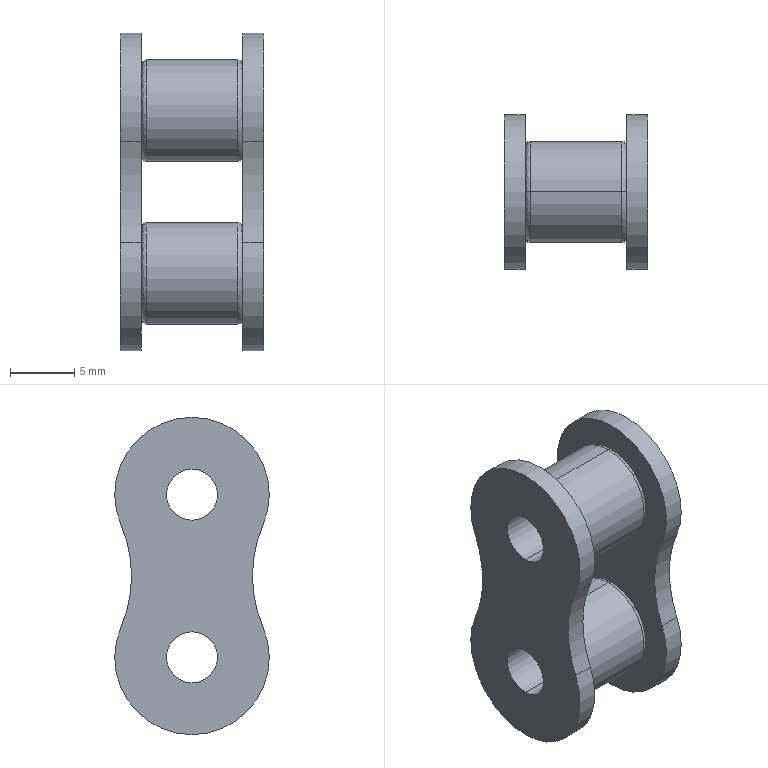Part | STEP file | 1.6 m_VMF01-40-4-A-002 | 1 solid | 30 faces | box 11.17 x 12.07 x 24.77 mm | volume 1310 mm3 | cylinder 18 | spline 8 | plane 4 | commonest cylinder face diameters 12.07 x6 3.98 x4 7.92 x4 20 x4
STEP:
#1=CARTESIAN_POINT('',(-3.56,0.,-3.96));
#2=VERTEX_POINT('',#1);
#3=CARTESIAN_POINT('',(-3.56,0.,3.96));
#4=VERTEX_POINT('',#3);
#5=CARTESIAN_POINT('',(-3.56,0.,0.));
#6=DIRECTION('',(-1.,0.,0.));
#7=DIRECTION('',(0.,0.,-1.));
#8=AXIS2_PLACEMENT_3D('',#5,#6,#7);
#9=CIRCLE('',#8,3.96);
#10=EDGE_CURVE('',#2,#4,#9,.T.);
#11=ORIENTED_EDGE('',*,*,#10,.T.);
#12=CARTESIAN_POINT('',(-3.96,0.,3.56));
#13=VERTEX_POINT('',#12);
#14=CARTESIAN_POINT('',(-3.56,0.,3.56));
#15=DIRECTION('',(0.,-1.,0.));
#16=DIRECTION('',(0.,0.,1.));
#17=AXIS2_PLACEMENT_3D('',#14,#15,#16);
#18=CIRCLE('',#17,0.4);
#19=EDGE_CURVE('',#4,#13,#18,.T.);
#20=ORIENTED_EDGE('',*,*,#19,.T.);
#21=CARTESIAN_POINT('',(-3.96,0.,-3.56));
#22=VERTEX_POINT('',#21);
#23=CARTESIAN_POINT('',(-3.96,0.,-3.56));
#24=CARTESIAN_POINT('',(-3.96,-0.2263,-3.56));
#25=CARTESIAN_POINT('',(-3.96,-0.5598,-3.529));
#26=CARTESIAN_POINT('',(-3.96,-0.9385,-3.438));
#27=CARTESIAN_POINT('',(-3.96,-1.125,-3.378));
#28=CARTESIAN_POINT('',(-3.96,-1.218,-3.345));
#29=CARTESIAN_POINT('',(-3.96,-1.258,-3.33));
#30=CARTESIAN_POINT('',(-3.96,-1.284,-3.32));
#31=CARTESIAN_POINT('',(-3.96,-1.296,-3.316));
#32=CARTESIAN_POINT('',(-3.96,-1.767,-3.129));
#33=CARTESIAN_POINT('',(-3.96,-2.17,-2.865));
#34=CARTESIAN_POINT('',(-3.96,-2.691,-2.344));
#35=CARTESIAN_POINT('',(-3.96,-2.92,-2.063));
#36=CARTESIAN_POINT('',(-3.96,-3.133,-1.699));
#37=CARTESIAN_POINT('',(-3.96,-3.226,-1.507));
#38=CARTESIAN_POINT('',(-3.96,-3.269,-1.41));
#39=CARTESIAN_POINT('',(-3.96,-3.287,-1.367));
#40=CARTESIAN_POINT('',(-3.96,-3.299,-1.339));
#41=CARTESIAN_POINT('',(-3.96,-3.305,-1.324));
#42=CARTESIAN_POINT('',(-3.96,-3.477,-0.8899));
#43=CARTESIAN_POINT('',(-3.96,-3.56,-0.4523));
#44=CARTESIAN_POINT('',(-3.96,-3.56,0.2262));
#45=CARTESIAN_POINT('',(-3.96,-3.529,0.5596));
#46=CARTESIAN_POINT('',(-3.96,-3.438,0.9384));
#47=CARTESIAN_POINT('',(-3.96,-3.378,1.125));
#48=CARTESIAN_POINT('',(-3.96,-3.345,1.218));
#49=CARTESIAN_POINT('',(-3.96,-3.33,1.258));
#50=CARTESIAN_POINT('',(-3.96,-3.32,1.284));
#51=CARTESIAN_POINT('',(-3.96,-3.316,1.296));
#52=CARTESIAN_POINT('',(-3.96,-3.129,1.767));
#53=CARTESIAN_POINT('',(-3.96,-2.865,2.17));
#54=CARTESIAN_POINT('',(-3.96,-2.344,2.691));
#55=CARTESIAN_POINT('',(-3.96,-2.063,2.92));
#56=CARTESIAN_POINT('',(-3.96,-1.699,3.133));
#57=CARTESIAN_POINT('',(-3.96,-1.507,3.226));
#58=CARTESIAN_POINT('',(-3.96,-1.41,3.269));
#59=CARTESIAN_POINT('',(-3.96,-1.367,3.287));
#60=CARTESIAN_POINT('',(-3.96,-1.339,3.299));
#61=CARTESIAN_POINT('',(-3.96,-1.324,3.305));
#62=CARTESIAN_POINT('',(-3.96,-0.8899,3.477));
#63=CARTESIAN_POINT('',(-3.96,-0.4523,3.56));
#64=CARTESIAN_POINT('',(-3.96,0.,3.56));
#65=B_SPLINE_CURVE_WITH_KNOTS('',3,(#23,#24,#25,#26,#27,#28,#29,#30,#31,#32,#33,#34,#35,#36,#37,#38,#39,#40,#41,#42,#43,#44,#45,#46,#47,#48,#49,#50,#51,#52,#53,#54,#55,#56,#57,#58,#59,#60,#61,#62,#63,#64),.UNSPECIFIED.,.F.,.F.,(4,1,1,1,1,2,2,2,1,1,1,1,2,2,2,1,1,1,1,2,2,2,1,1,1,1,2,2,4),(0.,0.03125,0.04687,0.05469,0.05859,0.06055,0.0625,0.125,0.1562,0.1719,0.1797,0.1836,0.1855,0.1875,0.25,0.2813,0.2969,0.3047,0.3086,0.3105,0.3125,0.375,0.4063,0.4219,0.4297,0.4336,0.4355,0.4375,0.5),.UNSPECIFIED.);
#66=EDGE_CURVE('',#22,#13,#65,.T.);
#67=ORIENTED_EDGE('',*,*,#66,.F.);
#68=CARTESIAN_POINT('',(-3.56,0.,-3.56));
#69=DIRECTION('',(0.,1.,0.));
#70=DIRECTION('',(0.,0.,-1.));
#71=AXIS2_PLACEMENT_3D('',#68,#69,#70);
#72=CIRCLE('',#71,0.4);
#73=EDGE_CURVE('',#2,#22,#72,.T.);
#74=ORIENTED_EDGE('',*,*,#73,.F.);
#75=EDGE_LOOP('',(#11,#20,#67,#74));
#76=FACE_OUTER_BOUND('',#75,.T.);
#77=CARTESIAN_POINT('',(-3.56,0.,3.96));
#78=CARTESIAN_POINT('',(-3.56,-7.92,3.96));
#79=CARTESIAN_POINT('',(-3.56,-7.92,-3.96));
#80=CARTESIAN_POINT('',(-3.56,0.,-3.96));
#81=CARTESIAN_POINT('',(-3.794,0.,3.96));
#82=CARTESIAN_POINT('',(-3.794,-7.92,3.96));
#83=CARTESIAN_POINT('',(-3.794,-7.92,-3.96));
#84=CARTESIAN_POINT('',(-3.794,0.,-3.96));
#85=CARTESIAN_POINT('',(-3.96,0.,3.794));
#86=CARTESIAN_POINT('',(-3.96,-7.589,3.794));
#87=CARTESIAN_POINT('',(-3.96,-7.589,-3.794));
#88=CARTESIAN_POINT('',(-3.96,0.,-3.794));
#89=CARTESIAN_POINT('',(-3.96,0.,3.56));
#90=CARTESIAN_POINT('',(-3.96,-7.12,3.56));
#91=CARTESIAN_POINT('',(-3.96,-7.12,-3.56));
#92=CARTESIAN_POINT('',(-3.96,0.,-3.56));
#93=(BOUNDED_SURFACE()B_SPLINE_SURFACE(3,3,((#77,#78,#79,#80),(#81,#82,#83,#84),(#85,#86,#87,#88),(#89,#90,#91,#92)),.UNSPECIFIED.,.F.,.F.,.F.)B_SPLINE_SURFACE_WITH_KNOTS((4,4),(4,4),(0.,1.),(0.,1.),.UNSPECIFIED.)GEOMETRIC_REPRESENTATION_ITEM()RATIONAL_B_SPLINE_SURFACE(((1.,0.3333,0.3333,1.),(0.8047,0.2682,0.2682,0.8047),(0.8047,0.2682,0.2682,0.8047),(1.,0.3333,0.3333,1.)))REPRESENTATION_ITEM('')SURFACE());
#94=ADVANCED_FACE('',(#76),#93,.T.);
#95=CARTESIAN_POINT('',(-3.56,0.,-16.66));
#96=VERTEX_POINT('',#95);
#97=CARTESIAN_POINT('',(-3.56,0.,-8.74));
#98=VERTEX_POINT('',#97);
#99=CARTESIAN_POINT('',(-3.56,0.,-12.7));
#100=DIRECTION('',(-1.,0.,0.));
#101=DIRECTION('',(0.,0.,-1.));
#102=AXIS2_PLACEMENT_3D('',#99,#100,#101);
#103=CIRCLE('',#102,3.96);
#104=EDGE_CURVE('',#96,#98,#103,.T.);
#105=ORIENTED_EDGE('',*,*,#104,.T.);
#106=CARTESIAN_POINT('',(-3.96,0.,-9.14));
#107=VERTEX_POINT('',#106);
#108=CARTESIAN_POINT('',(-3.56,0.,-9.14));
#109=DIRECTION('',(0.,-1.,0.));
#110=DIRECTION('',(0.,0.,1.));
#111=AXIS2_PLACEMENT_3D('',#108,#109,#110);
#112=CIRCLE('',#111,0.4);
#113=EDGE_CURVE('',#98,#107,#112,.T.);
#114=ORIENTED_EDGE('',*,*,#113,.T.);
#115=CARTESIAN_POINT('',(-3.96,0.,-16.26));
#116=VERTEX_POINT('',#115);
#117=CARTESIAN_POINT('',(-3.96,0.,-16.26));
#118=CARTESIAN_POINT('',(-3.96,-0.2263,-16.26));
#119=CARTESIAN_POINT('',(-3.96,-0.5598,-16.229));
#120=CARTESIAN_POINT('',(-3.96,-0.9385,-16.138));
#121=CARTESIAN_POINT('',(-3.96,-1.125,-16.078));
#122=CARTESIAN_POINT('',(-3.96,-1.218,-16.045));
#123=CARTESIAN_POINT('',(-3.96,-1.258,-16.03));
#124=CARTESIAN_POINT('',(-3.96,-1.284,-16.02));
#125=CARTESIAN_POINT('',(-3.96,-1.296,-16.016));
#126=CARTESIAN_POINT('',(-3.96,-1.767,-15.829));
#127=CARTESIAN_POINT('',(-3.96,-2.17,-15.565));
#128=CARTESIAN_POINT('',(-3.96,-2.691,-15.044));
#129=CARTESIAN_POINT('',(-3.96,-2.92,-14.763));
#130=CARTESIAN_POINT('',(-3.96,-3.133,-14.399));
#131=CARTESIAN_POINT('',(-3.96,-3.226,-14.207));
#132=CARTESIAN_POINT('',(-3.96,-3.269,-14.11));
#133=CARTESIAN_POINT('',(-3.96,-3.287,-14.067));
#134=CARTESIAN_POINT('',(-3.96,-3.299,-14.039));
#135=CARTESIAN_POINT('',(-3.96,-3.305,-14.024));
#136=CARTESIAN_POINT('',(-3.96,-3.477,-13.59));
#137=CARTESIAN_POINT('',(-3.96,-3.56,-13.152));
#138=CARTESIAN_POINT('',(-3.96,-3.56,-12.474));
#139=CARTESIAN_POINT('',(-3.96,-3.529,-12.14));
#140=CARTESIAN_POINT('',(-3.96,-3.438,-11.762));
#141=CARTESIAN_POINT('',(-3.96,-3.378,-11.575));
#142=CARTESIAN_POINT('',(-3.96,-3.345,-11.482));
#143=CARTESIAN_POINT('',(-3.96,-3.33,-11.442));
#144=CARTESIAN_POINT('',(-3.96,-3.32,-11.416));
#145=CARTESIAN_POINT('',(-3.96,-3.316,-11.404));
#146=CARTESIAN_POINT('',(-3.96,-3.129,-10.933));
#147=CARTESIAN_POINT('',(-3.96,-2.865,-10.53));
#148=CARTESIAN_POINT('',(-3.96,-2.344,-10.009));
#149=CARTESIAN_POINT('',(-3.96,-2.063,-9.78));
#150=CARTESIAN_POINT('',(-3.96,-1.699,-9.567));
#151=CARTESIAN_POINT('',(-3.96,-1.507,-9.474));
#152=CARTESIAN_POINT('',(-3.96,-1.41,-9.431));
#153=CARTESIAN_POINT('',(-3.96,-1.367,-9.413));
#154=CARTESIAN_POINT('',(-3.96,-1.339,-9.401));
#155=CARTESIAN_POINT('',(-3.96,-1.324,-9.395));
#156=CARTESIAN_POINT('',(-3.96,-0.8899,-9.223));
#157=CARTESIAN_POINT('',(-3.96,-0.4523,-9.14));
#158=CARTESIAN_POINT('',(-3.96,0.,-9.14));
#159=B_SPLINE_CURVE_WITH_KNOTS('',3,(#117,#118,#119,#120,#121,#122,#123,#124,#125,#126,#127,#128,#129,#130,#131,#132,#133,#134,#135,#136,#137,#138,#139,#140,#141,#142,#143,#144,#145,#146,#147,#148,#149,#150,#151,#152,#153,#154,#155,#156,#157,#158),.UNSPECIFIED.,.F.,.F.,(4,1,1,1,1,2,2,2,1,1,1,1,2,2,2,1,1,1,1,2,2,2,1,1,1,1,2,2,4),(0.,0.03125,0.04688,0.05469,0.05859,0.06055,0.0625,0.125,0.1562,0.1719,0.1797,0.1836,0.1855,0.1875,0.25,0.2812,0.2969,0.3047,0.3086,0.3105,0.3125,0.375,0.4062,0.4219,0.4297,0.4336,0.4355,0.4375,0.5),.UNSPECIFIED.);
#160=EDGE_CURVE('',#116,#107,#159,.T.);
#161=ORIENTED_EDGE('',*,*,#160,.F.);
#162=CARTESIAN_POINT('',(-3.56,0.,-16.26));
#163=DIRECTION('',(0.,1.,0.));
#164=DIRECTION('',(0.,0.,-1.));
#165=AXIS2_PLACEMENT_3D('',#162,#163,#164);
#166=CIRCLE('',#165,0.4);
#167=EDGE_CURVE('',#96,#116,#166,.T.);
#168=ORIENTED_EDGE('',*,*,#167,.F.);
#169=EDGE_LOOP('',(#105,#114,#161,#168));
#170=FACE_OUTER_BOUND('',#169,.T.);
#171=CARTESIAN_POINT('',(-3.56,0.,-8.74));
#172=CARTESIAN_POINT('',(-3.56,-7.92,-8.74));
#173=CARTESIAN_POINT('',(-3.56,-7.92,-16.66));
#174=CARTESIAN_POINT('',(-3.56,0.,-16.66));
#175=CARTESIAN_POINT('',(-3.794,0.,-8.74));
#176=CARTESIAN_POINT('',(-3.794,-7.92,-8.74));
#177=CARTESIAN_POINT('',(-3.794,-7.92,-16.66));
#178=CARTESIAN_POINT('',(-3.794,0.,-16.66));
#179=CARTESIAN_POINT('',(-3.96,0.,-8.906));
#180=CARTESIAN_POINT('',(-3.96,-7.589,-8.906));
#181=CARTESIAN_POINT('',(-3.96,-7.589,-16.494));
#182=CARTESIAN_POINT('',(-3.96,0.,-16.494));
#183=CARTESIAN_POINT('',(-3.96,0.,-9.14));
#184=CARTESIAN_POINT('',(-3.96,-7.12,-9.14));
#185=CARTESIAN_POINT('',(-3.96,-7.12,-16.26));
#186=CARTESIAN_POINT('',(-3.96,0.,-16.26));
#187=(BOUNDED_SURFACE()B_SPLINE_SURFACE(3,3,((#171,#172,#173,#174),(#175,#176,#177,#178),(#179,#180,#181,#182),(#183,#184,#185,#186)),.UNSPECIFIED.,.F.,.F.,.F.)B_SPLINE_SURFACE_WITH_KNOTS((4,4),(4,4),(0.,1.),(0.,1.),.UNSPECIFIED.)GEOMETRIC_REPRESENTATION_ITEM()RATIONAL_B_SPLINE_SURFACE(((1.,0.3333,0.3333,1.),(0.8047,0.2682,0.2682,0.8047),(0.8047,0.2682,0.2682,0.8047),(1.,0.3333,0.3333,1.)))REPRESENTATION_ITEM('')SURFACE());
#188=ADVANCED_FACE('',(#170),#187,.T.);
#189=CARTESIAN_POINT('',(3.96,0.,-3.56));
#190=VERTEX_POINT('',#189);
#191=CARTESIAN_POINT('',(3.96,0.,3.56));
#192=VERTEX_POINT('',#191);
#193=CARTESIAN_POINT('',(3.96,0.,-3.56));
#194=CARTESIAN_POINT('',(3.96,-7.12,-3.56));
#195=CARTESIAN_POINT('',(3.96,-7.12,3.56));
#196=CARTESIAN_POINT('',(3.96,0.,3.56));
#197=(BOUNDED_CURVE()B_SPLINE_CURVE(3,(#193,#194,#195,#196),.UNSPECIFIED.,.F.,.F.)B_SPLINE_CURVE_WITH_KNOTS((4,4),(0.,0.5),.UNSPECIFIED.)CURVE()GEOMETRIC_REPRESENTATION_ITEM()RATIONAL_B_SPLINE_CURVE((1.,0.3333,0.3333,1.))REPRESENTATION_ITEM(''));
#198=EDGE_CURVE('',#190,#192,#197,.T.);
#199=ORIENTED_EDGE('',*,*,#198,.T.);
#200=CARTESIAN_POINT('',(3.56,0.,3.96));
#201=VERTEX_POINT('',#200);
#202=CARTESIAN_POINT('',(3.56,0.,3.56));
#203=DIRECTION('',(0.,-1.,0.));
#204=DIRECTION('',(0.,0.,1.));
#205=AXIS2_PLACEMENT_3D('',#202,#203,#204);
#206=CIRCLE('',#205,0.4);
#207=EDGE_CURVE('',#192,#201,#206,.T.);
#208=ORIENTED_EDGE('',*,*,#207,.T.);
#209=CARTESIAN_POINT('',(3.56,0.,-3.96));
#210=VERTEX_POINT('',#209);
#211=CARTESIAN_POINT('',(3.56,0.,0.));
#212=DIRECTION('',(-1.,0.,0.));
#213=DIRECTION('',(0.,0.,1.));
#214=AXIS2_PLACEMENT_3D('',#211,#212,#213);
#215=CIRCLE('',#214,3.96);
#216=EDGE_CURVE('',#210,#201,#215,.T.);
#217=ORIENTED_EDGE('',*,*,#216,.F.);
#218=CARTESIAN_POINT('',(3.56,0.,-3.56));
#219=DIRECTION('',(0.,1.,0.));
#220=DIRECTION('',(0.,0.,-1.));
#221=AXIS2_PLACEMENT_3D('',#218,#219,#220);
#222=CIRCLE('',#221,0.4);
#223=EDGE_CURVE('',#190,#210,#222,.T.);
#224=ORIENTED_EDGE('',*,*,#223,.F.);
#225=EDGE_LOOP('',(#199,#208,#217,#224));
#226=FACE_OUTER_BOUND('',#225,.T.);
#227=CARTESIAN_POINT('',(3.96,0.,3.56));
#228=CARTESIAN_POINT('',(3.96,-7.12,3.56));
#229=CARTESIAN_POINT('',(3.96,-7.12,-3.56));
#230=CARTESIAN_POINT('',(3.96,0.,-3.56));
#231=CARTESIAN_POINT('',(3.96,0.,3.794));
#232=CARTESIAN_POINT('',(3.96,-7.589,3.794));
#233=CARTESIAN_POINT('',(3.96,-7.589,-3.794));
#234=CARTESIAN_POINT('',(3.96,0.,-3.794));
#235=CARTESIAN_POINT('',(3.794,0.,3.96));
#236=CARTESIAN_POINT('',(3.794,-7.92,3.96));
#237=CARTESIAN_POINT('',(3.794,-7.92,-3.96));
#238=CARTESIAN_POINT('',(3.794,0.,-3.96));
#239=CARTESIAN_POINT('',(3.56,0.,3.96));
#240=CARTESIAN_POINT('',(3.56,-7.92,3.96));
#241=CARTESIAN_POINT('',(3.56,-7.92,-3.96));
#242=CARTESIAN_POINT('',(3.56,0.,-3.96));
#243=(BOUNDED_SURFACE()B_SPLINE_SURFACE(3,3,((#227,#228,#229,#230),(#231,#232,#233,#234),(#235,#236,#237,#238),(#239,#240,#241,#242)),.UNSPECIFIED.,.F.,.F.,.F.)B_SPLINE_SURFACE_WITH_KNOTS((4,4),(4,4),(0.,1.),(0.,1.),.UNSPECIFIED.)GEOMETRIC_REPRESENTATION_ITEM()RATIONAL_B_SPLINE_SURFACE(((1.,0.3333,0.3333,1.),(0.8047,0.2682,0.2682,0.8047),(0.8047,0.2682,0.2682,0.8047),(1.,0.3333,0.3333,1.)))REPRESENTATION_ITEM('')SURFACE());
#244=ADVANCED_FACE('',(#226),#243,.T.);
#245=CARTESIAN_POINT('',(3.96,0.,-16.26));
#246=VERTEX_POINT('',#245);
#247=CARTESIAN_POINT('',(3.96,0.,-9.14));
#248=VERTEX_POINT('',#247);
#249=CARTESIAN_POINT('',(3.96,0.,-16.26));
#250=CARTESIAN_POINT('',(3.96,-7.12,-16.26));
#251=CARTESIAN_POINT('',(3.96,-7.12,-9.14));
#252=CARTESIAN_POINT('',(3.96,0.,-9.14));
#253=(BOUNDED_CURVE()B_SPLINE_CURVE(3,(#249,#250,#251,#252),.UNSPECIFIED.,.F.,.F.)B_SPLINE_CURVE_WITH_KNOTS((4,4),(0.,0.5),.UNSPECIFIED.)CURVE()GEOMETRIC_REPRESENTATION_ITEM()RATIONAL_B_SPLINE_CURVE((1.,0.3333,0.3333,1.))REPRESENTATION_ITEM(''));
#254=EDGE_CURVE('',#246,#248,#253,.T.);
#255=ORIENTED_EDGE('',*,*,#254,.T.);
#256=CARTESIAN_POINT('',(3.56,0.,-8.74));
#257=VERTEX_POINT('',#256);
#258=CARTESIAN_POINT('',(3.56,0.,-9.14));
#259=DIRECTION('',(0.,-1.,0.));
#260=DIRECTION('',(0.,0.,1.));
#261=AXIS2_PLACEMENT_3D('',#258,#259,#260);
#262=CIRCLE('',#261,0.4);
#263=EDGE_CURVE('',#248,#257,#262,.T.);
#264=ORIENTED_EDGE('',*,*,#263,.T.);
#265=CARTESIAN_POINT('',(3.56,0.,-16.66));
#266=VERTEX_POINT('',#265);
#267=CARTESIAN_POINT('',(3.56,0.,-12.7));
#268=DIRECTION('',(-1.,0.,0.));
#269=DIRECTION('',(0.,0.,1.));
#270=AXIS2_PLACEMENT_3D('',#267,#268,#269);
#271=CIRCLE('',#270,3.96);
#272=EDGE_CURVE('',#266,#257,#271,.T.);
#273=ORIENTED_EDGE('',*,*,#272,.F.);
#274=CARTESIAN_POINT('',(3.56,0.,-16.26));
#275=DIRECTION('',(0.,1.,0.));
#276=DIRECTION('',(0.,0.,-1.));
#277=AXIS2_PLACEMENT_3D('',#274,#275,#276);
#278=CIRCLE('',#277,0.4);
#279=EDGE_CURVE('',#246,#266,#278,.T.);
#280=ORIENTED_EDGE('',*,*,#279,.F.);
#281=EDGE_LOOP('',(#255,#264,#273,#280));
#282=FACE_OUTER_BOUND('',#281,.T.);
#283=CARTESIAN_POINT('',(3.96,0.,-9.14));
#284=CARTESIAN_POINT('',(3.96,-7.12,-9.14));
#285=CARTESIAN_POINT('',(3.96,-7.12,-16.26));
#286=CARTESIAN_POINT('',(3.96,0.,-16.26));
#287=CARTESIAN_POINT('',(3.96,0.,-8.906));
#288=CARTESIAN_POINT('',(3.96,-7.589,-8.906));
#289=CARTESIAN_POINT('',(3.96,-7.589,-16.494));
#290=CARTESIAN_POINT('',(3.96,0.,-16.494));
#291=CARTESIAN_POINT('',(3.794,0.,-8.74));
#292=CARTESIAN_POINT('',(3.794,-7.92,-8.74));
#293=CARTESIAN_POINT('',(3.794,-7.92,-16.66));
#294=CARTESIAN_POINT('',(3.794,0.,-16.66));
#295=CARTESIAN_POINT('',(3.56,0.,-8.74));
#296=CARTESIAN_POINT('',(3.56,-7.92,-8.74));
#297=CARTESIAN_POINT('',(3.56,-7.92,-16.66));
#298=CARTESIAN_POINT('',(3.56,0.,-16.66));
#299=(BOUNDED_SURFACE()B_SPLINE_SURFACE(3,3,((#283,#284,#285,#286),(#287,#288,#289,#290),(#291,#292,#293,#294),(#295,#296,#297,#298)),.UNSPECIFIED.,.F.,.F.,.F.)B_SPLINE_SURFACE_WITH_KNOTS((4,4),(4,4),(0.,1.),(0.,1.),.UNSPECIFIED.)GEOMETRIC_REPRESENTATION_ITEM()RATIONAL_B_SPLINE_SURFACE(((1.,0.3333,0.3333,1.),(0.8047,0.2682,0.2682,0.8047),(0.8047,0.2682,0.2682,0.8047),(1.,0.3333,0.3333,1.)))REPRESENTATION_ITEM('')SURFACE());
#300=ADVANCED_FACE('',(#282),#299,.T.);
#301=CARTESIAN_POINT('',(-5.585,0.,-1.99));
#302=VERTEX_POINT('',#301);
#303=CARTESIAN_POINT('',(-5.585,0.,1.99));
#304=VERTEX_POINT('',#303);
#305=CARTESIAN_POINT('',(-5.585,0.,0.));
#306=DIRECTION('',(-1.,0.,0.));
#307=DIRECTION('',(0.,0.,-1.));
#308=AXIS2_PLACEMENT_3D('',#305,#306,#307);
#309=CIRCLE('',#308,1.99);
#310=EDGE_CURVE('',#302,#304,#309,.T.);
#311=ORIENTED_EDGE('',*,*,#310,.T.);
#312=CARTESIAN_POINT('',(5.585,0.,1.99));
#313=VERTEX_POINT('',#312);
#314=CARTESIAN_POINT('',(5.585,0.,1.99));
#315=DIRECTION('',(1.,0.,0.));
#316=VECTOR('',#315,1000.);
#317=LINE('',#314,#316);
#318=EDGE_CURVE('',#304,#313,#317,.T.);
#319=ORIENTED_EDGE('',*,*,#318,.T.);
#320=CARTESIAN_POINT('',(5.585,0.,-1.99));
#321=VERTEX_POINT('',#320);
#322=CARTESIAN_POINT('',(5.585,0.,0.));
#323=DIRECTION('',(-1.,0.,0.));
#324=DIRECTION('',(0.,0.,-1.));
#325=AXIS2_PLACEMENT_3D('',#322,#323,#324);
#326=CIRCLE('',#325,1.99);
#327=EDGE_CURVE('',#321,#313,#326,.T.);
#328=ORIENTED_EDGE('',*,*,#327,.F.);
#329=CARTESIAN_POINT('',(5.585,0.,-1.99));
#330=DIRECTION('',(1.,0.,0.));
#331=VECTOR('',#330,1000.);
#332=LINE('',#329,#331);
#333=EDGE_CURVE('',#302,#321,#332,.T.);
#334=ORIENTED_EDGE('',*,*,#333,.F.);
#335=EDGE_LOOP('',(#311,#319,#328,#334));
#336=FACE_OUTER_BOUND('',#335,.T.);
#337=CARTESIAN_POINT('',(5.585,0.,0.));
#338=DIRECTION('',(1.,0.,0.));
#339=DIRECTION('',(0.,0.,-1.));
#340=AXIS2_PLACEMENT_3D('',#337,#338,#339);
#341=CYLINDRICAL_SURFACE('',#340,1.99);
#342=ADVANCED_FACE('',(#336),#341,.F.);
#343=CARTESIAN_POINT('',(-5.585,-5.542,-10.31));
#344=VERTEX_POINT('',#343);
#345=CARTESIAN_POINT('',(-5.585,0.,-18.735));
#346=VERTEX_POINT('',#345);
#347=CARTESIAN_POINT('',(-5.585,0.,-12.7));
#348=DIRECTION('',(1.,0.,0.));
#349=DIRECTION('',(0.,0.,-1.));
#350=AXIS2_PLACEMENT_3D('',#347,#348,#349);
#351=CIRCLE('',#350,6.035);
#352=EDGE_CURVE('',#344,#346,#351,.T.);
#353=ORIENTED_EDGE('',*,*,#352,.T.);
#354=CARTESIAN_POINT('',(-3.96,0.,-18.735));
#355=VERTEX_POINT('',#354);
#356=CARTESIAN_POINT('',(5.585,0.,-18.735));
#357=DIRECTION('',(1.,0.,0.));
#358=VECTOR('',#357,1000.);
#359=LINE('',#356,#358);
#360=EDGE_CURVE('',#346,#355,#359,.T.);
#361=ORIENTED_EDGE('',*,*,#360,.T.);
#362=CARTESIAN_POINT('',(-3.96,-5.542,-10.31));
#363=VERTEX_POINT('',#362);
#364=CARTESIAN_POINT('',(-3.96,0.,-12.7));
#365=DIRECTION('',(-1.,0.,0.));
#366=DIRECTION('',(0.,0.,-1.));
#367=AXIS2_PLACEMENT_3D('',#364,#365,#366);
#368=CIRCLE('',#367,6.035);
#369=EDGE_CURVE('',#355,#363,#368,.T.);
#370=ORIENTED_EDGE('',*,*,#369,.T.);
#371=CARTESIAN_POINT('',(5.585,-5.542,-10.31));
#372=DIRECTION('',(-1.,0.,0.));
#373=VECTOR('',#372,1000.);
#374=LINE('',#371,#373);
#375=EDGE_CURVE('',#363,#344,#374,.T.);
#376=ORIENTED_EDGE('',*,*,#375,.T.);
#377=EDGE_LOOP('',(#353,#361,#370,#376));
#378=FACE_OUTER_BOUND('',#377,.T.);
#379=CARTESIAN_POINT('',(5.585,0.,-12.7));
#380=DIRECTION('',(1.,0.,0.));
#381=DIRECTION('',(0.,0.,-1.));
#382=AXIS2_PLACEMENT_3D('',#379,#380,#381);
#383=CYLINDRICAL_SURFACE('',#382,6.035);
#384=ADVANCED_FACE('',(#378),#383,.T.);
#385=CARTESIAN_POINT('',(-5.585,0.,-14.69));
#386=VERTEX_POINT('',#385);
#387=CARTESIAN_POINT('',(-5.585,0.,-10.71));
#388=VERTEX_POINT('',#387);
#389=CARTESIAN_POINT('',(-5.585,0.,-12.7));
#390=DIRECTION('',(-1.,0.,0.));
#391=DIRECTION('',(0.,0.,-1.));
#392=AXIS2_PLACEMENT_3D('',#389,#390,#391);
#393=CIRCLE('',#392,1.99);
#394=EDGE_CURVE('',#386,#388,#393,.T.);
#395=ORIENTED_EDGE('',*,*,#394,.T.);
#396=CARTESIAN_POINT('',(5.585,0.,-10.71));
#397=VERTEX_POINT('',#396);
#398=CARTESIAN_POINT('',(5.585,0.,-10.71));
#399=DIRECTION('',(1.,0.,0.));
#400=VECTOR('',#399,1000.);
#401=LINE('',#398,#400);
#402=EDGE_CURVE('',#388,#397,#401,.T.);
#403=ORIENTED_EDGE('',*,*,#402,.T.);
#404=CARTESIAN_POINT('',(5.585,0.,-14.69));
#405=VERTEX_POINT('',#404);
#406=CARTESIAN_POINT('',(5.585,0.,-12.7));
#407=DIRECTION('',(-1.,0.,0.));
#408=DIRECTION('',(0.,0.,-1.));
#409=AXIS2_PLACEMENT_3D('',#406,#407,#408);
#410=CIRCLE('',#409,1.99);
#411=EDGE_CURVE('',#405,#397,#410,.T.);
#412=ORIENTED_EDGE('',*,*,#411,.F.);
#413=CARTESIAN_POINT('',(5.585,0.,-14.69));
#414=DIRECTION('',(1.,0.,0.));
#415=VECTOR('',#414,1000.);
#416=LINE('',#413,#415);
#417=EDGE_CURVE('',#386,#405,#416,.T.);
#418=ORIENTED_EDGE('',*,*,#417,.F.);
#419=EDGE_LOOP('',(#395,#403,#412,#418));
#420=FACE_OUTER_BOUND('',#419,.T.);
#421=CARTESIAN_POINT('',(5.585,0.,-12.7));
#422=DIRECTION('',(1.,0.,0.));
#423=DIRECTION('',(0.,0.,-1.));
#424=AXIS2_PLACEMENT_3D('',#421,#422,#423);
#425=CYLINDRICAL_SURFACE('',#424,1.99);
#426=ADVANCED_FACE('',(#420),#425,.F.);
#427=CARTESIAN_POINT('',(3.96,-5.542,-10.31));
#428=VERTEX_POINT('',#427);
#429=CARTESIAN_POINT('',(3.96,0.,-18.735));
#430=VERTEX_POINT('',#429);
#431=CARTESIAN_POINT('',(3.96,0.,-12.7));
#432=DIRECTION('',(1.,0.,0.));
#433=DIRECTION('',(0.,0.,-1.));
#434=AXIS2_PLACEMENT_3D('',#431,#432,#433);
#435=CIRCLE('',#434,6.035);
#436=EDGE_CURVE('',#428,#430,#435,.T.);
#437=ORIENTED_EDGE('',*,*,#436,.T.);
#438=CARTESIAN_POINT('',(5.585,0.,-18.735));
#439=VERTEX_POINT('',#438);
#440=CARTESIAN_POINT('',(5.585,0.,-18.735));
#441=DIRECTION('',(1.,0.,0.));
#442=VECTOR('',#441,1000.);
#443=LINE('',#440,#442);
#444=EDGE_CURVE('',#430,#439,#443,.T.);
#445=ORIENTED_EDGE('',*,*,#444,.T.);
#446=CARTESIAN_POINT('',(5.585,-5.542,-10.31));
#447=VERTEX_POINT('',#446);
#448=CARTESIAN_POINT('',(5.585,0.,-12.7));
#449=DIRECTION('',(1.,0.,0.));
#450=DIRECTION('',(0.,0.,-1.));
#451=AXIS2_PLACEMENT_3D('',#448,#449,#450);
#452=CIRCLE('',#451,6.035);
#453=EDGE_CURVE('',#447,#439,#452,.T.);
#454=ORIENTED_EDGE('',*,*,#453,.F.);
#455=CARTESIAN_POINT('',(5.585,-5.542,-10.31));
#456=DIRECTION('',(-1.,0.,0.));
#457=VECTOR('',#456,1000.);
#458=LINE('',#455,#457);
#459=EDGE_CURVE('',#447,#428,#458,.T.);
#460=ORIENTED_EDGE('',*,*,#459,.T.);
#461=EDGE_LOOP('',(#437,#445,#454,#460));
#462=FACE_OUTER_BOUND('',#461,.T.);
#463=CARTESIAN_POINT('',(5.585,0.,-12.7));
#464=DIRECTION('',(1.,0.,0.));
#465=DIRECTION('',(0.,0.,-1.));
#466=AXIS2_PLACEMENT_3D('',#463,#464,#465);
#467=CYLINDRICAL_SURFACE('',#466,6.035);
#468=ADVANCED_FACE('',(#462),#467,.T.);
#469=CARTESIAN_POINT('',(3.56,0.,0.));
#470=DIRECTION('',(-1.,0.,0.));
#471=DIRECTION('',(0.,0.,1.));
#472=AXIS2_PLACEMENT_3D('',#469,#470,#471);
#473=CIRCLE('',#472,3.96);
#474=EDGE_CURVE('',#201,#210,#473,.T.);
#475=ORIENTED_EDGE('',*,*,#474,.T.);
#476=CARTESIAN_POINT('',(50.,0.,-3.96));
#477=DIRECTION('',(-1.,0.,0.));
#478=VECTOR('',#477,1000.);
#479=LINE('',#476,#478);
#480=EDGE_CURVE('',#210,#2,#479,.T.);
#481=ORIENTED_EDGE('',*,*,#480,.T.);
#482=CARTESIAN_POINT('',(-3.56,0.,0.));
#483=DIRECTION('',(-1.,0.,0.));
#484=DIRECTION('',(0.,0.,-1.));
#485=AXIS2_PLACEMENT_3D('',#482,#483,#484);
#486=CIRCLE('',#485,3.96);
#487=EDGE_CURVE('',#4,#2,#486,.T.);
#488=ORIENTED_EDGE('',*,*,#487,.F.);
#489=CARTESIAN_POINT('',(50.,0.,3.96));
#490=DIRECTION('',(-1.,0.,0.));
#491=VECTOR('',#490,1000.);
#492=LINE('',#489,#491);
#493=EDGE_CURVE('',#201,#4,#492,.T.);
#494=ORIENTED_EDGE('',*,*,#493,.F.);
#495=EDGE_LOOP('',(#475,#481,#488,#494));
#496=FACE_OUTER_BOUND('',#495,.T.);
#497=CARTESIAN_POINT('',(50.,0.,0.));
#498=DIRECTION('',(-1.,0.,0.));
#499=DIRECTION('',(0.,0.,1.));
#500=AXIS2_PLACEMENT_3D('',#497,#498,#499);
#501=CYLINDRICAL_SURFACE('',#500,3.96);
#502=ADVANCED_FACE('',(#496),#501,.T.);
#503=CARTESIAN_POINT('',(3.56,0.,-12.7));
#504=DIRECTION('',(-1.,0.,0.));
#505=DIRECTION('',(0.,0.,1.));
#506=AXIS2_PLACEMENT_3D('',#503,#504,#505);
#507=CIRCLE('',#506,3.96);
#508=EDGE_CURVE('',#257,#266,#507,.T.);
#509=ORIENTED_EDGE('',*,*,#508,.T.);
#510=CARTESIAN_POINT('',(50.,0.,-16.66));
#511=DIRECTION('',(-1.,0.,0.));
#512=VECTOR('',#511,1000.);
#513=LINE('',#510,#512);
#514=EDGE_CURVE('',#266,#96,#513,.T.);
#515=ORIENTED_EDGE('',*,*,#514,.T.);
#516=CARTESIAN_POINT('',(-3.56,0.,-12.7));
#517=DIRECTION('',(-1.,0.,0.));
#518=DIRECTION('',(0.,0.,-1.));
#519=AXIS2_PLACEMENT_3D('',#516,#517,#518);
#520=CIRCLE('',#519,3.96);
#521=EDGE_CURVE('',#98,#96,#520,.T.);
#522=ORIENTED_EDGE('',*,*,#521,.F.);
#523=CARTESIAN_POINT('',(50.,0.,-8.74));
#524=DIRECTION('',(-1.,0.,0.));
#525=VECTOR('',#524,1000.);
#526=LINE('',#523,#525);
#527=EDGE_CURVE('',#257,#98,#526,.T.);
#528=ORIENTED_EDGE('',*,*,#527,.F.);
#529=EDGE_LOOP('',(#509,#515,#522,#528));
#530=FACE_OUTER_BOUND('',#529,.T.);
#531=CARTESIAN_POINT('',(50.,0.,-12.7));
#532=DIRECTION('',(-1.,0.,0.));
#533=DIRECTION('',(0.,0.,1.));
#534=AXIS2_PLACEMENT_3D('',#531,#532,#533);
#535=CYLINDRICAL_SURFACE('',#534,3.96);
#536=ADVANCED_FACE('',(#530),#535,.T.);
#537=ORIENTED_EDGE('',*,*,#310,.F.);
#538=CARTESIAN_POINT('',(-5.585,0.,0.));
#539=DIRECTION('',(-1.,0.,0.));
#540=DIRECTION('',(0.,0.,-1.));
#541=AXIS2_PLACEMENT_3D('',#538,#539,#540);
#542=CIRCLE('',#541,1.99);
#543=EDGE_CURVE('',#304,#302,#542,.T.);
#544=ORIENTED_EDGE('',*,*,#543,.F.);
#545=EDGE_LOOP('',(#537,#544));
#546=FACE_BOUND('',#545,.T.);
#547=ORIENTED_EDGE('',*,*,#352,.F.);
#548=CARTESIAN_POINT('',(-5.585,-5.542,-2.39));
#549=VERTEX_POINT('',#548);
#550=CARTESIAN_POINT('',(-5.585,-14.724,-6.35));
#551=DIRECTION('',(-1.,0.,0.));
#552=DIRECTION('',(0.,0.,-1.));
#553=AXIS2_PLACEMENT_3D('',#550,#551,#552);
#554=CIRCLE('',#553,10.);
#555=EDGE_CURVE('',#549,#344,#554,.T.);
#556=ORIENTED_EDGE('',*,*,#555,.F.);
#557=CARTESIAN_POINT('',(-5.585,5.542,-2.39));
#558=VERTEX_POINT('',#557);
#559=CARTESIAN_POINT('',(-5.585,0.,0.));
#560=DIRECTION('',(1.,0.,0.));
#561=DIRECTION('',(0.,0.,-1.));
#562=AXIS2_PLACEMENT_3D('',#559,#560,#561);
#563=CIRCLE('',#562,6.035);
#564=EDGE_CURVE('',#558,#549,#563,.T.);
#565=ORIENTED_EDGE('',*,*,#564,.F.);
#566=CARTESIAN_POINT('',(-5.585,5.542,-10.31));
#567=VERTEX_POINT('',#566);
#568=CARTESIAN_POINT('',(-5.585,14.724,-6.35));
#569=DIRECTION('',(-1.,0.,0.));
#570=DIRECTION('',(0.,0.,-1.));
#571=AXIS2_PLACEMENT_3D('',#568,#569,#570);
#572=CIRCLE('',#571,10.);
#573=EDGE_CURVE('',#567,#558,#572,.T.);
#574=ORIENTED_EDGE('',*,*,#573,.F.);
#575=CARTESIAN_POINT('',(-5.585,0.,-12.7));
#576=DIRECTION('',(1.,0.,0.));
#577=DIRECTION('',(0.,0.,-1.));
#578=AXIS2_PLACEMENT_3D('',#575,#576,#577);
#579=CIRCLE('',#578,6.035);
#580=EDGE_CURVE('',#346,#567,#579,.T.);
#581=ORIENTED_EDGE('',*,*,#580,.F.);
#582=EDGE_LOOP('',(#547,#556,#565,#574,#581));
#583=FACE_OUTER_BOUND('',#582,.T.);
#584=ORIENTED_EDGE('',*,*,#394,.F.);
#585=CARTESIAN_POINT('',(-5.585,0.,-12.7));
#586=DIRECTION('',(-1.,0.,0.));
#587=DIRECTION('',(0.,0.,-1.));
#588=AXIS2_PLACEMENT_3D('',#585,#586,#587);
#589=CIRCLE('',#588,1.99);
#590=EDGE_CURVE('',#388,#386,#589,.T.);
#591=ORIENTED_EDGE('',*,*,#590,.F.);
#592=EDGE_LOOP('',(#584,#591));
#593=FACE_BOUND('',#592,.T.);
#594=CARTESIAN_POINT('',(-5.585,7.362,-9.525));
#595=DIRECTION('',(1.,0.,0.));
#596=DIRECTION('',(0.,0.,-1.));
#597=AXIS2_PLACEMENT_3D('',#594,#595,#596);
#598=PLANE('',#597);
#599=ADVANCED_FACE('',(#546,#583,#593),#598,.F.);
#600=ORIENTED_EDGE('',*,*,#318,.F.);
#601=ORIENTED_EDGE('',*,*,#543,.T.);
#602=ORIENTED_EDGE('',*,*,#333,.T.);
#603=CARTESIAN_POINT('',(5.585,0.,0.));
#604=DIRECTION('',(-1.,0.,0.));
#605=DIRECTION('',(0.,0.,-1.));
#606=AXIS2_PLACEMENT_3D('',#603,#604,#605);
#607=CIRCLE('',#606,1.99);
#608=EDGE_CURVE('',#313,#321,#607,.T.);
#609=ORIENTED_EDGE('',*,*,#608,.F.);
#610=EDGE_LOOP('',(#600,#601,#602,#609));
#611=FACE_OUTER_BOUND('',#610,.T.);
#612=CARTESIAN_POINT('',(5.585,0.,0.));
#613=DIRECTION('',(1.,0.,0.));
#614=DIRECTION('',(0.,0.,-1.));
#615=AXIS2_PLACEMENT_3D('',#612,#613,#614);
#616=CYLINDRICAL_SURFACE('',#615,1.99);
#617=ADVANCED_FACE('',(#611),#616,.F.);
#618=CARTESIAN_POINT('',(-3.96,5.542,-10.31));
#619=VERTEX_POINT('',#618);
#620=CARTESIAN_POINT('',(-3.96,5.542,-2.39));
#621=VERTEX_POINT('',#620);
#622=CARTESIAN_POINT('',(-3.96,14.724,-6.35));
#623=DIRECTION('',(-1.,0.,0.));
#624=DIRECTION('',(0.,0.,-1.));
#625=AXIS2_PLACEMENT_3D('',#622,#623,#624);
#626=CIRCLE('',#625,10.);
#627=EDGE_CURVE('',#619,#621,#626,.T.);
#628=ORIENTED_EDGE('',*,*,#627,.F.);
#629=CARTESIAN_POINT('',(5.585,5.542,-10.31));
#630=DIRECTION('',(1.,0.,0.));
#631=VECTOR('',#630,1000.);
#632=LINE('',#629,#631);
#633=EDGE_CURVE('',#567,#619,#632,.T.);
#634=ORIENTED_EDGE('',*,*,#633,.F.);
#635=ORIENTED_EDGE('',*,*,#573,.T.);
#636=CARTESIAN_POINT('',(5.585,5.542,-2.39));
#637=DIRECTION('',(-1.,0.,0.));
#638=VECTOR('',#637,1000.);
#639=LINE('',#636,#638);
#640=EDGE_CURVE('',#621,#558,#639,.T.);
#641=ORIENTED_EDGE('',*,*,#640,.F.);
#642=EDGE_LOOP('',(#628,#634,#635,#641));
#643=FACE_OUTER_BOUND('',#642,.T.);
#644=CARTESIAN_POINT('',(5.585,14.724,-6.35));
#645=DIRECTION('',(1.,0.,0.));
#646=DIRECTION('',(0.,0.,-1.));
#647=AXIS2_PLACEMENT_3D('',#644,#645,#646);
#648=CYLINDRICAL_SURFACE('',#647,10.);
#649=ADVANCED_FACE('',(#643),#648,.F.);
#650=ORIENTED_EDGE('',*,*,#360,.F.);
#651=ORIENTED_EDGE('',*,*,#580,.T.);
#652=ORIENTED_EDGE('',*,*,#633,.T.);
#653=CARTESIAN_POINT('',(-3.96,0.,-12.7));
#654=DIRECTION('',(-1.,0.,0.));
#655=DIRECTION('',(0.,0.,-1.));
#656=AXIS2_PLACEMENT_3D('',#653,#654,#655);
#657=CIRCLE('',#656,6.035);
#658=EDGE_CURVE('',#619,#355,#657,.T.);
#659=ORIENTED_EDGE('',*,*,#658,.T.);
#660=EDGE_LOOP('',(#650,#651,#652,#659));
#661=FACE_OUTER_BOUND('',#660,.T.);
#662=CARTESIAN_POINT('',(5.585,0.,-12.7));
#663=DIRECTION('',(1.,0.,0.));
#664=DIRECTION('',(0.,0.,-1.));
#665=AXIS2_PLACEMENT_3D('',#662,#663,#664);
#666=CYLINDRICAL_SURFACE('',#665,6.035);
#667=ADVANCED_FACE('',(#661),#666,.T.);
#668=CARTESIAN_POINT('',(-3.96,-5.542,-2.39));
#669=VERTEX_POINT('',#668);
#670=CARTESIAN_POINT('',(-3.96,-14.724,-6.35));
#671=DIRECTION('',(-1.,0.,0.));
#672=DIRECTION('',(0.,0.,-1.));
#673=AXIS2_PLACEMENT_3D('',#670,#671,#672);
#674=CIRCLE('',#673,10.);
#675=EDGE_CURVE('',#669,#363,#674,.T.);
#676=ORIENTED_EDGE('',*,*,#675,.F.);
#677=CARTESIAN_POINT('',(5.585,-5.542,-2.39));
#678=DIRECTION('',(1.,0.,0.));
#679=VECTOR('',#678,1000.);
#680=LINE('',#677,#679);
#681=EDGE_CURVE('',#549,#669,#680,.T.);
#682=ORIENTED_EDGE('',*,*,#681,.F.);
#683=ORIENTED_EDGE('',*,*,#555,.T.);
#684=ORIENTED_EDGE('',*,*,#375,.F.);
#685=EDGE_LOOP('',(#676,#682,#683,#684));
#686=FACE_OUTER_BOUND('',#685,.T.);
#687=CARTESIAN_POINT('',(5.585,-14.724,-6.35));
#688=DIRECTION('',(1.,0.,0.));
#689=DIRECTION('',(0.,0.,-1.));
#690=AXIS2_PLACEMENT_3D('',#687,#688,#689);
#691=CYLINDRICAL_SURFACE('',#690,10.);
#692=ADVANCED_FACE('',(#686),#691,.F.);
#693=ORIENTED_EDGE('',*,*,#564,.T.);
#694=ORIENTED_EDGE('',*,*,#681,.T.);
#695=CARTESIAN_POINT('',(-3.96,0.,0.));
#696=DIRECTION('',(-1.,0.,0.));
#697=DIRECTION('',(0.,0.,-1.));
#698=AXIS2_PLACEMENT_3D('',#695,#696,#697);
#699=CIRCLE('',#698,6.035);
#700=EDGE_CURVE('',#669,#621,#699,.T.);
#701=ORIENTED_EDGE('',*,*,#700,.T.);
#702=ORIENTED_EDGE('',*,*,#640,.T.);
#703=EDGE_LOOP('',(#693,#694,#701,#702));
#704=FACE_OUTER_BOUND('',#703,.T.);
#705=CARTESIAN_POINT('',(5.585,0.,0.));
#706=DIRECTION('',(1.,0.,0.));
#707=DIRECTION('',(0.,0.,-1.));
#708=AXIS2_PLACEMENT_3D('',#705,#706,#707);
#709=CYLINDRICAL_SURFACE('',#708,6.035);
#710=ADVANCED_FACE('',(#704),#709,.T.);
#711=ORIENTED_EDGE('',*,*,#402,.F.);
#712=ORIENTED_EDGE('',*,*,#590,.T.);
#713=ORIENTED_EDGE('',*,*,#417,.T.);
#714=CARTESIAN_POINT('',(5.585,0.,-12.7));
#715=DIRECTION('',(-1.,0.,0.));
#716=DIRECTION('',(0.,0.,-1.));
#717=AXIS2_PLACEMENT_3D('',#714,#715,#716);
#718=CIRCLE('',#717,1.99);
#719=EDGE_CURVE('',#397,#405,#718,.T.);
#720=ORIENTED_EDGE('',*,*,#719,.F.);
#721=EDGE_LOOP('',(#711,#712,#713,#720));
#722=FACE_OUTER_BOUND('',#721,.T.);
#723=CARTESIAN_POINT('',(5.585,0.,-12.7));
#724=DIRECTION('',(1.,0.,0.));
#725=DIRECTION('',(0.,0.,-1.));
#726=AXIS2_PLACEMENT_3D('',#723,#724,#725);
#727=CYLINDRICAL_SURFACE('',#726,1.99);
#728=ADVANCED_FACE('',(#722),#727,.F.);
#729=ORIENTED_EDGE('',*,*,#327,.T.);
#730=ORIENTED_EDGE('',*,*,#608,.T.);
#731=EDGE_LOOP('',(#729,#730));
#732=FACE_BOUND('',#731,.T.);
#733=CARTESIAN_POINT('',(5.585,-5.542,-2.39));
#734=VERTEX_POINT('',#733);
#735=CARTESIAN_POINT('',(5.585,-14.724,-6.35));
#736=DIRECTION('',(-1.,0.,0.));
#737=DIRECTION('',(0.,0.,-1.));
#738=AXIS2_PLACEMENT_3D('',#735,#736,#737);
#739=CIRCLE('',#738,10.);
#740=EDGE_CURVE('',#734,#447,#739,.T.);
#741=ORIENTED_EDGE('',*,*,#740,.T.);
#742=ORIENTED_EDGE('',*,*,#453,.T.);
#743=CARTESIAN_POINT('',(5.585,5.542,-10.31));
#744=VERTEX_POINT('',#743);
#745=CARTESIAN_POINT('',(5.585,0.,-12.7));
#746=DIRECTION('',(1.,0.,0.));
#747=DIRECTION('',(0.,0.,-1.));
#748=AXIS2_PLACEMENT_3D('',#745,#746,#747);
#749=CIRCLE('',#748,6.035);
#750=EDGE_CURVE('',#439,#744,#749,.T.);
#751=ORIENTED_EDGE('',*,*,#750,.T.);
#752=CARTESIAN_POINT('',(5.585,5.542,-2.39));
#753=VERTEX_POINT('',#752);
#754=CARTESIAN_POINT('',(5.585,14.724,-6.35));
#755=DIRECTION('',(-1.,0.,0.));
#756=DIRECTION('',(0.,0.,-1.));
#757=AXIS2_PLACEMENT_3D('',#754,#755,#756);
#758=CIRCLE('',#757,10.);
#759=EDGE_CURVE('',#744,#753,#758,.T.);
#760=ORIENTED_EDGE('',*,*,#759,.T.);
#761=CARTESIAN_POINT('',(5.585,0.,0.));
#762=DIRECTION('',(1.,0.,0.));
#763=DIRECTION('',(0.,0.,-1.));
#764=AXIS2_PLACEMENT_3D('',#761,#762,#763);
#765=CIRCLE('',#764,6.035);
#766=EDGE_CURVE('',#753,#734,#765,.T.);
#767=ORIENTED_EDGE('',*,*,#766,.T.);
#768=EDGE_LOOP('',(#741,#742,#751,#760,#767));
#769=FACE_OUTER_BOUND('',#768,.T.);
#770=ORIENTED_EDGE('',*,*,#411,.T.);
#771=ORIENTED_EDGE('',*,*,#719,.T.);
#772=EDGE_LOOP('',(#770,#771));
#773=FACE_BOUND('',#772,.T.);
#774=CARTESIAN_POINT('',(5.585,7.362,-9.525));
#775=DIRECTION('',(1.,0.,0.));
#776=DIRECTION('',(0.,0.,-1.));
#777=AXIS2_PLACEMENT_3D('',#774,#775,#776);
#778=PLANE('',#777);
#779=ADVANCED_FACE('',(#732,#769,#773),#778,.T.);
#780=ORIENTED_EDGE('',*,*,#675,.T.);
#781=ORIENTED_EDGE('',*,*,#369,.F.);
#782=ORIENTED_EDGE('',*,*,#658,.F.);
#783=ORIENTED_EDGE('',*,*,#627,.T.);
#784=ORIENTED_EDGE('',*,*,#700,.F.);
#785=EDGE_LOOP('',(#780,#781,#782,#783,#784));
#786=FACE_OUTER_BOUND('',#785,.T.);
#787=ORIENTED_EDGE('',*,*,#66,.T.);
#788=CARTESIAN_POINT('',(-3.96,0.,3.56));
#789=CARTESIAN_POINT('',(-3.96,0.2262,3.56));
#790=CARTESIAN_POINT('',(-3.96,0.5596,3.529));
#791=CARTESIAN_POINT('',(-3.96,0.9384,3.438));
#792=CARTESIAN_POINT('',(-3.96,1.125,3.378));
#793=CARTESIAN_POINT('',(-3.96,1.218,3.345));
#794=CARTESIAN_POINT('',(-3.96,1.258,3.33));
#795=CARTESIAN_POINT('',(-3.96,1.284,3.32));
#796=CARTESIAN_POINT('',(-3.96,1.296,3.316));
#797=CARTESIAN_POINT('',(-3.96,1.767,3.129));
#798=CARTESIAN_POINT('',(-3.96,2.17,2.865));
#799=CARTESIAN_POINT('',(-3.96,2.691,2.344));
#800=CARTESIAN_POINT('',(-3.96,2.92,2.063));
#801=CARTESIAN_POINT('',(-3.96,3.133,1.699));
#802=CARTESIAN_POINT('',(-3.96,3.226,1.507));
#803=CARTESIAN_POINT('',(-3.96,3.269,1.41));
#804=CARTESIAN_POINT('',(-3.96,3.287,1.367));
#805=CARTESIAN_POINT('',(-3.96,3.299,1.339));
#806=CARTESIAN_POINT('',(-3.96,3.305,1.324));
#807=CARTESIAN_POINT('',(-3.96,3.477,0.8899));
#808=CARTESIAN_POINT('',(-3.96,3.56,0.4523));
#809=CARTESIAN_POINT('',(-3.96,3.56,-0.2262));
#810=CARTESIAN_POINT('',(-3.96,3.529,-0.5596));
#811=CARTESIAN_POINT('',(-3.96,3.438,-0.9384));
#812=CARTESIAN_POINT('',(-3.96,3.378,-1.125));
#813=CARTESIAN_POINT('',(-3.96,3.345,-1.218));
#814=CARTESIAN_POINT('',(-3.96,3.33,-1.258));
#815=CARTESIAN_POINT('',(-3.96,3.32,-1.284));
#816=CARTESIAN_POINT('',(-3.96,3.316,-1.296));
#817=CARTESIAN_POINT('',(-3.96,3.129,-1.767));
#818=CARTESIAN_POINT('',(-3.96,2.865,-2.17));
#819=CARTESIAN_POINT('',(-3.96,2.344,-2.691));
#820=CARTESIAN_POINT('',(-3.96,2.063,-2.92));
#821=CARTESIAN_POINT('',(-3.96,1.699,-3.133));
#822=CARTESIAN_POINT('',(-3.96,1.507,-3.226));
#823=CARTESIAN_POINT('',(-3.96,1.41,-3.269));
#824=CARTESIAN_POINT('',(-3.96,1.367,-3.287));
#825=CARTESIAN_POINT('',(-3.96,1.339,-3.299));
#826=CARTESIAN_POINT('',(-3.96,1.324,-3.305));
#827=CARTESIAN_POINT('',(-3.96,0.8897,-3.477));
#828=CARTESIAN_POINT('',(-3.96,0.4529,-3.56));
#829=CARTESIAN_POINT('',(-3.96,0.,-3.56));
#830=B_SPLINE_CURVE_WITH_KNOTS('',3,(#788,#789,#790,#791,#792,#793,#794,#795,#796,#797,#798,#799,#800,#801,#802,#803,#804,#805,#806,#807,#808,#809,#810,#811,#812,#813,#814,#815,#816,#817,#818,#819,#820,#821,#822,#823,#824,#825,#826,#827,#828,#829),.UNSPECIFIED.,.F.,.F.,(4,1,1,1,1,2,2,2,1,1,1,1,2,2,2,1,1,1,1,2,2,2,1,1,1,1,2,2,4),(0.5,0.5313,0.5469,0.5547,0.5586,0.5605,0.5625,0.625,0.6563,0.6719,0.6797,0.6836,0.6855,0.6875,0.75,0.7813,0.7969,0.8047,0.8086,0.8105,0.8125,0.875,0.9063,0.9219,0.9297,0.9336,0.9355,0.9375,1.),.UNSPECIFIED.);
#831=EDGE_CURVE('',#13,#22,#830,.T.);
#832=ORIENTED_EDGE('',*,*,#831,.T.);
#833=EDGE_LOOP('',(#787,#832));
#834=FACE_BOUND('',#833,.T.);
#835=ORIENTED_EDGE('',*,*,#160,.T.);
#836=CARTESIAN_POINT('',(-3.96,0.,-9.14));
#837=CARTESIAN_POINT('',(-3.96,0.2262,-9.14));
#838=CARTESIAN_POINT('',(-3.96,0.5596,-9.171));
#839=CARTESIAN_POINT('',(-3.96,0.9384,-9.262));
#840=CARTESIAN_POINT('',(-3.96,1.125,-9.322));
#841=CARTESIAN_POINT('',(-3.96,1.218,-9.355));
#842=CARTESIAN_POINT('',(-3.96,1.258,-9.37));
#843=CARTESIAN_POINT('',(-3.96,1.284,-9.38));
#844=CARTESIAN_POINT('',(-3.96,1.296,-9.384));
#845=CARTESIAN_POINT('',(-3.96,1.767,-9.571));
#846=CARTESIAN_POINT('',(-3.96,2.17,-9.835));
#847=CARTESIAN_POINT('',(-3.96,2.691,-10.356));
#848=CARTESIAN_POINT('',(-3.96,2.92,-10.637));
#849=CARTESIAN_POINT('',(-3.96,3.133,-11.001));
#850=CARTESIAN_POINT('',(-3.96,3.226,-11.193));
#851=CARTESIAN_POINT('',(-3.96,3.269,-11.29));
#852=CARTESIAN_POINT('',(-3.96,3.287,-11.333));
#853=CARTESIAN_POINT('',(-3.96,3.299,-11.361));
#854=CARTESIAN_POINT('',(-3.96,3.305,-11.376));
#855=CARTESIAN_POINT('',(-3.96,3.477,-11.81));
#856=CARTESIAN_POINT('',(-3.96,3.56,-12.248));
#857=CARTESIAN_POINT('',(-3.96,3.56,-12.926));
#858=CARTESIAN_POINT('',(-3.96,3.529,-13.26));
#859=CARTESIAN_POINT('',(-3.96,3.438,-13.638));
#860=CARTESIAN_POINT('',(-3.96,3.378,-13.825));
#861=CARTESIAN_POINT('',(-3.96,3.345,-13.918));
#862=CARTESIAN_POINT('',(-3.96,3.33,-13.958));
#863=CARTESIAN_POINT('',(-3.96,3.32,-13.984));
#864=CARTESIAN_POINT('',(-3.96,3.316,-13.996));
#865=CARTESIAN_POINT('',(-3.96,3.129,-14.467));
#866=CARTESIAN_POINT('',(-3.96,2.865,-14.87));
#867=CARTESIAN_POINT('',(-3.96,2.344,-15.391));
#868=CARTESIAN_POINT('',(-3.96,2.063,-15.62));
#869=CARTESIAN_POINT('',(-3.96,1.699,-15.833));
#870=CARTESIAN_POINT('',(-3.96,1.507,-15.926));
#871=CARTESIAN_POINT('',(-3.96,1.41,-15.969));
#872=CARTESIAN_POINT('',(-3.96,1.367,-15.987));
#873=CARTESIAN_POINT('',(-3.96,1.339,-15.999));
#874=CARTESIAN_POINT('',(-3.96,1.324,-16.005));
#875=CARTESIAN_POINT('',(-3.96,0.8897,-16.177));
#876=CARTESIAN_POINT('',(-3.96,0.4529,-16.26));
#877=CARTESIAN_POINT('',(-3.96,0.,-16.26));
#878=B_SPLINE_CURVE_WITH_KNOTS('',3,(#836,#837,#838,#839,#840,#841,#842,#843,#844,#845,#846,#847,#848,#849,#850,#851,#852,#853,#854,#855,#856,#857,#858,#859,#860,#861,#862,#863,#864,#865,#866,#867,#868,#869,#870,#871,#872,#873,#874,#875,#876,#877),.UNSPECIFIED.,.F.,.F.,(4,1,1,1,1,2,2,2,1,1,1,1,2,2,2,1,1,1,1,2,2,2,1,1,1,1,2,2,4),(0.5,0.5312,0.5469,0.5547,0.5586,0.5605,0.5625,0.625,0.6562,0.6719,0.6797,0.6836,0.6855,0.6875,0.75,0.7812,0.7969,0.8047,0.8086,0.8105,0.8125,0.875,0.9062,0.9219,0.9297,0.9336,0.9355,0.9375,1.),.UNSPECIFIED.);
#879=EDGE_CURVE('',#107,#116,#878,.T.);
#880=ORIENTED_EDGE('',*,*,#879,.T.);
#881=EDGE_LOOP('',(#835,#880));
#882=FACE_BOUND('',#881,.T.);
#883=CARTESIAN_POINT('',(-3.96,7.362,-9.525));
#884=DIRECTION('',(1.,0.,0.));
#885=DIRECTION('',(0.,0.,-1.));
#886=AXIS2_PLACEMENT_3D('',#883,#884,#885);
#887=PLANE('',#886);
#888=ADVANCED_FACE('',(#786,#834,#882),#887,.T.);
#889=ORIENTED_EDGE('',*,*,#444,.F.);
#890=CARTESIAN_POINT('',(3.96,5.542,-10.31));
#891=VERTEX_POINT('',#890);
#892=CARTESIAN_POINT('',(3.96,0.,-12.7));
#893=DIRECTION('',(1.,0.,0.));
#894=DIRECTION('',(0.,0.,-1.));
#895=AXIS2_PLACEMENT_3D('',#892,#893,#894);
#896=CIRCLE('',#895,6.035);
#897=EDGE_CURVE('',#430,#891,#896,.T.);
#898=ORIENTED_EDGE('',*,*,#897,.T.);
#899=CARTESIAN_POINT('',(5.585,5.542,-10.31));
#900=DIRECTION('',(1.,0.,0.));
#901=VECTOR('',#900,1000.);
#902=LINE('',#899,#901);
#903=EDGE_CURVE('',#891,#744,#902,.T.);
#904=ORIENTED_EDGE('',*,*,#903,.T.);
#905=ORIENTED_EDGE('',*,*,#750,.F.);
#906=EDGE_LOOP('',(#889,#898,#904,#905));
#907=FACE_OUTER_BOUND('',#906,.T.);
#908=CARTESIAN_POINT('',(5.585,0.,-12.7));
#909=DIRECTION('',(1.,0.,0.));
#910=DIRECTION('',(0.,0.,-1.));
#911=AXIS2_PLACEMENT_3D('',#908,#909,#910);
#912=CYLINDRICAL_SURFACE('',#911,6.035);
#913=ADVANCED_FACE('',(#907),#912,.T.);
#914=ORIENTED_EDGE('',*,*,#459,.F.);
#915=ORIENTED_EDGE('',*,*,#740,.F.);
#916=CARTESIAN_POINT('',(3.96,-5.542,-2.39));
#917=VERTEX_POINT('',#916);
#918=CARTESIAN_POINT('',(5.585,-5.542,-2.39));
#919=DIRECTION('',(1.,0.,0.));
#920=VECTOR('',#919,1000.);
#921=LINE('',#918,#920);
#922=EDGE_CURVE('',#917,#734,#921,.T.);
#923=ORIENTED_EDGE('',*,*,#922,.F.);
#924=CARTESIAN_POINT('',(3.96,-14.724,-6.35));
#925=DIRECTION('',(1.,0.,0.));
#926=DIRECTION('',(0.,0.,-1.));
#927=AXIS2_PLACEMENT_3D('',#924,#925,#926);
#928=CIRCLE('',#927,10.);
#929=EDGE_CURVE('',#428,#917,#928,.T.);
#930=ORIENTED_EDGE('',*,*,#929,.F.);
#931=EDGE_LOOP('',(#914,#915,#923,#930));
#932=FACE_OUTER_BOUND('',#931,.T.);
#933=CARTESIAN_POINT('',(5.585,-14.724,-6.35));
#934=DIRECTION('',(1.,0.,0.));
#935=DIRECTION('',(0.,0.,-1.));
#936=AXIS2_PLACEMENT_3D('',#933,#934,#935);
#937=CYLINDRICAL_SURFACE('',#936,10.);
#938=ADVANCED_FACE('',(#932),#937,.F.);
#939=ORIENTED_EDGE('',*,*,#922,.T.);
#940=ORIENTED_EDGE('',*,*,#766,.F.);
#941=CARTESIAN_POINT('',(3.96,5.542,-2.39));
#942=VERTEX_POINT('',#941);
#943=CARTESIAN_POINT('',(5.585,5.542,-2.39));
#944=DIRECTION('',(-1.,0.,0.));
#945=VECTOR('',#944,1000.);
#946=LINE('',#943,#945);
#947=EDGE_CURVE('',#753,#942,#946,.T.);
#948=ORIENTED_EDGE('',*,*,#947,.T.);
#949=CARTESIAN_POINT('',(3.96,0.,0.));
#950=DIRECTION('',(1.,0.,0.));
#951=DIRECTION('',(0.,0.,-1.));
#952=AXIS2_PLACEMENT_3D('',#949,#950,#951);
#953=CIRCLE('',#952,6.035);
#954=EDGE_CURVE('',#942,#917,#953,.T.);
#955=ORIENTED_EDGE('',*,*,#954,.T.);
#956=EDGE_LOOP('',(#939,#940,#948,#955));
#957=FACE_OUTER_BOUND('',#956,.T.);
#958=CARTESIAN_POINT('',(5.585,0.,0.));
#959=DIRECTION('',(1.,0.,0.));
#960=DIRECTION('',(0.,0.,-1.));
#961=AXIS2_PLACEMENT_3D('',#958,#959,#960);
#962=CYLINDRICAL_SURFACE('',#961,6.035);
#963=ADVANCED_FACE('',(#957),#962,.T.);
#964=ORIENTED_EDGE('',*,*,#947,.F.);
#965=ORIENTED_EDGE('',*,*,#759,.F.);
#966=ORIENTED_EDGE('',*,*,#903,.F.);
#967=CARTESIAN_POINT('',(3.96,14.724,-6.35));
#968=DIRECTION('',(1.,0.,0.));
#969=DIRECTION('',(0.,0.,-1.));
#970=AXIS2_PLACEMENT_3D('',#967,#968,#969);
#971=CIRCLE('',#970,10.);
#972=EDGE_CURVE('',#942,#891,#971,.T.);
#973=ORIENTED_EDGE('',*,*,#972,.F.);
#974=EDGE_LOOP('',(#964,#965,#966,#973));
#975=FACE_OUTER_BOUND('',#974,.T.);
#976=CARTESIAN_POINT('',(5.585,14.724,-6.35));
#977=DIRECTION('',(1.,0.,0.));
#978=DIRECTION('',(0.,0.,-1.));
#979=AXIS2_PLACEMENT_3D('',#976,#977,#978);
#980=CYLINDRICAL_SURFACE('',#979,10.);
#981=ADVANCED_FACE('',(#975),#980,.F.);
#982=ORIENTED_EDGE('',*,*,#19,.F.);
#983=ORIENTED_EDGE('',*,*,#487,.T.);
#984=ORIENTED_EDGE('',*,*,#73,.T.);
#985=ORIENTED_EDGE('',*,*,#831,.F.);
#986=EDGE_LOOP('',(#982,#983,#984,#985));
#987=FACE_OUTER_BOUND('',#986,.T.);
#988=CARTESIAN_POINT('',(-3.56,0.,-3.96));
#989=CARTESIAN_POINT('',(-3.56,7.92,-3.96));
#990=CARTESIAN_POINT('',(-3.56,7.92,3.96));
#991=CARTESIAN_POINT('',(-3.56,0.,3.96));
#992=CARTESIAN_POINT('',(-3.794,0.,-3.96));
#993=CARTESIAN_POINT('',(-3.794,7.92,-3.96));
#994=CARTESIAN_POINT('',(-3.794,7.92,3.96));
#995=CARTESIAN_POINT('',(-3.794,0.,3.96));
#996=CARTESIAN_POINT('',(-3.96,0.,-3.794));
#997=CARTESIAN_POINT('',(-3.96,7.589,-3.794));
#998=CARTESIAN_POINT('',(-3.96,7.589,3.794));
#999=CARTESIAN_POINT('',(-3.96,0.,3.794));
#1000=CARTESIAN_POINT('',(-3.96,0.,-3.56));
#1001=CARTESIAN_POINT('',(-3.96,7.12,-3.56));
#1002=CARTESIAN_POINT('',(-3.96,7.12,3.56));
#1003=CARTESIAN_POINT('',(-3.96,0.,3.56));
#1004=(BOUNDED_SURFACE()B_SPLINE_SURFACE(3,3,((#988,#989,#990,#991),(#992,#993,#994,#995),(#996,#997,#998,#999),(#1000,#1001,#1002,#1003)),.UNSPECIFIED.,.F.,.F.,.T.)B_SPLINE_SURFACE_WITH_KNOTS((4,4),(4,4),(0.,1.),(0.,1.),.UNSPECIFIED.)GEOMETRIC_REPRESENTATION_ITEM()RATIONAL_B_SPLINE_SURFACE(((1.,0.3333,0.3333,1.),(0.8047,0.2682,0.2682,0.8047),(0.8047,0.2682,0.2682,0.8047),(1.,0.3333,0.3333,1.)))REPRESENTATION_ITEM('')SURFACE());
#1005=ADVANCED_FACE('',(#987),#1004,.T.);
#1006=ORIENTED_EDGE('',*,*,#113,.F.);
#1007=ORIENTED_EDGE('',*,*,#521,.T.);
#1008=ORIENTED_EDGE('',*,*,#167,.T.);
#1009=ORIENTED_EDGE('',*,*,#879,.F.);
#1010=EDGE_LOOP('',(#1006,#1007,#1008,#1009));
#1011=FACE_OUTER_BOUND('',#1010,.T.);
#1012=CARTESIAN_POINT('',(-3.56,0.,-16.66));
#1013=CARTESIAN_POINT('',(-3.56,7.92,-16.66));
#1014=CARTESIAN_POINT('',(-3.56,7.92,-8.74));
#1015=CARTESIAN_POINT('',(-3.56,0.,-8.74));
#1016=CARTESIAN_POINT('',(-3.794,0.,-16.66));
#1017=CARTESIAN_POINT('',(-3.794,7.92,-16.66));
#1018=CARTESIAN_POINT('',(-3.794,7.92,-8.74));
#1019=CARTESIAN_POINT('',(-3.794,0.,-8.74));
#1020=CARTESIAN_POINT('',(-3.96,0.,-16.494));
#1021=CARTESIAN_POINT('',(-3.96,7.589,-16.494));
#1022=CARTESIAN_POINT('',(-3.96,7.589,-8.906));
#1023=CARTESIAN_POINT('',(-3.96,0.,-8.906));
#1024=CARTESIAN_POINT('',(-3.96,0.,-16.26));
#1025=CARTESIAN_POINT('',(-3.96,7.12,-16.26));
#1026=CARTESIAN_POINT('',(-3.96,7.12,-9.14));
#1027=CARTESIAN_POINT('',(-3.96,0.,-9.14));
#1028=(BOUNDED_SURFACE()B_SPLINE_SURFACE(3,3,((#1012,#1013,#1014,#1015),(#1016,#1017,#1018,#1019),(#1020,#1021,#1022,#1023),(#1024,#1025,#1026,#1027)),.UNSPECIFIED.,.F.,.F.,.F.)B_SPLINE_SURFACE_WITH_KNOTS((4,4),(4,4),(0.,1.),(0.,1.),.UNSPECIFIED.)GEOMETRIC_REPRESENTATION_ITEM()RATIONAL_B_SPLINE_SURFACE(((1.,0.3333,0.3333,1.),(0.8047,0.2682,0.2682,0.8047),(0.8047,0.2682,0.2682,0.8047),(1.,0.3333,0.3333,1.)))REPRESENTATION_ITEM('')SURFACE());
#1029=ADVANCED_FACE('',(#1011),#1028,.T.);
#1030=ORIENTED_EDGE('',*,*,#436,.F.);
#1031=ORIENTED_EDGE('',*,*,#929,.T.);
#1032=ORIENTED_EDGE('',*,*,#954,.F.);
#1033=ORIENTED_EDGE('',*,*,#972,.T.);
#1034=ORIENTED_EDGE('',*,*,#897,.F.);
#1035=EDGE_LOOP('',(#1030,#1031,#1032,#1033,#1034));
#1036=FACE_OUTER_BOUND('',#1035,.T.);
#1037=ORIENTED_EDGE('',*,*,#198,.F.);
#1038=CARTESIAN_POINT('',(3.96,0.,3.56));
#1039=CARTESIAN_POINT('',(3.96,7.12,3.56));
#1040=CARTESIAN_POINT('',(3.96,7.12,-3.56));
#1041=CARTESIAN_POINT('',(3.96,0.,-3.56));
#1042=(BOUNDED_CURVE()B_SPLINE_CURVE(3,(#1038,#1039,#1040,#1041),.UNSPECIFIED.,.F.,.F.)B_SPLINE_CURVE_WITH_KNOTS((4,4),(0.5,1.),.UNSPECIFIED.)CURVE()GEOMETRIC_REPRESENTATION_ITEM()RATIONAL_B_SPLINE_CURVE((1.,0.3333,0.3333,1.))REPRESENTATION_ITEM(''));
#1043=EDGE_CURVE('',#192,#190,#1042,.T.);
#1044=ORIENTED_EDGE('',*,*,#1043,.F.);
#1045=EDGE_LOOP('',(#1037,#1044));
#1046=FACE_BOUND('',#1045,.T.);
#1047=ORIENTED_EDGE('',*,*,#254,.F.);
#1048=CARTESIAN_POINT('',(3.96,0.,-9.14));
#1049=CARTESIAN_POINT('',(3.96,7.12,-9.14));
#1050=CARTESIAN_POINT('',(3.96,7.12,-16.26));
#1051=CARTESIAN_POINT('',(3.96,0.,-16.26));
#1052=(BOUNDED_CURVE()B_SPLINE_CURVE(3,(#1048,#1049,#1050,#1051),.UNSPECIFIED.,.F.,.T.)B_SPLINE_CURVE_WITH_KNOTS((4,4),(0.5,1.),.UNSPECIFIED.)CURVE()GEOMETRIC_REPRESENTATION_ITEM()RATIONAL_B_SPLINE_CURVE((1.,0.3333,0.3333,1.))REPRESENTATION_ITEM(''));
#1053=EDGE_CURVE('',#248,#246,#1052,.T.);
#1054=ORIENTED_EDGE('',*,*,#1053,.F.);
#1055=EDGE_LOOP('',(#1047,#1054));
#1056=FACE_BOUND('',#1055,.T.);
#1057=CARTESIAN_POINT('',(3.96,7.362,-9.525));
#1058=DIRECTION('',(1.,0.,0.));
#1059=DIRECTION('',(0.,0.,-1.));
#1060=AXIS2_PLACEMENT_3D('',#1057,#1058,#1059);
#1061=PLANE('',#1060);
#1062=ADVANCED_FACE('',(#1036,#1046,#1056),#1061,.F.);
#1063=ORIENTED_EDGE('',*,*,#480,.F.);
#1064=ORIENTED_EDGE('',*,*,#216,.T.);
#1065=ORIENTED_EDGE('',*,*,#493,.T.);
#1066=ORIENTED_EDGE('',*,*,#10,.F.);
#1067=EDGE_LOOP('',(#1063,#1064,#1065,#1066));
#1068=FACE_OUTER_BOUND('',#1067,.T.);
#1069=CARTESIAN_POINT('',(50.,0.,0.));
#1070=DIRECTION('',(-1.,0.,0.));
#1071=DIRECTION('',(0.,0.,1.));
#1072=AXIS2_PLACEMENT_3D('',#1069,#1070,#1071);
#1073=CYLINDRICAL_SURFACE('',#1072,3.96);
#1074=ADVANCED_FACE('',(#1068),#1073,.T.);
#1075=ORIENTED_EDGE('',*,*,#514,.F.);
#1076=ORIENTED_EDGE('',*,*,#272,.T.);
#1077=ORIENTED_EDGE('',*,*,#527,.T.);
#1078=ORIENTED_EDGE('',*,*,#104,.F.);
#1079=EDGE_LOOP('',(#1075,#1076,#1077,#1078));
#1080=FACE_OUTER_BOUND('',#1079,.T.);
#1081=CARTESIAN_POINT('',(50.,0.,-12.7));
#1082=DIRECTION('',(-1.,0.,0.));
#1083=DIRECTION('',(0.,0.,1.));
#1084=AXIS2_PLACEMENT_3D('',#1081,#1082,#1083);
#1085=CYLINDRICAL_SURFACE('',#1084,3.96);
#1086=ADVANCED_FACE('',(#1080),#1085,.T.);
#1087=ORIENTED_EDGE('',*,*,#207,.F.);
#1088=ORIENTED_EDGE('',*,*,#1043,.T.);
#1089=ORIENTED_EDGE('',*,*,#223,.T.);
#1090=ORIENTED_EDGE('',*,*,#474,.F.);
#1091=EDGE_LOOP('',(#1087,#1088,#1089,#1090));
#1092=FACE_OUTER_BOUND('',#1091,.T.);
#1093=CARTESIAN_POINT('',(3.96,0.,-3.56));
#1094=CARTESIAN_POINT('',(3.96,7.12,-3.56));
#1095=CARTESIAN_POINT('',(3.96,7.12,3.56));
#1096=CARTESIAN_POINT('',(3.96,0.,3.56));
#1097=CARTESIAN_POINT('',(3.96,0.,-3.794));
#1098=CARTESIAN_POINT('',(3.96,7.589,-3.794));
#1099=CARTESIAN_POINT('',(3.96,7.589,3.794));
#1100=CARTESIAN_POINT('',(3.96,0.,3.794));
#1101=CARTESIAN_POINT('',(3.794,0.,-3.96));
#1102=CARTESIAN_POINT('',(3.794,7.92,-3.96));
#1103=CARTESIAN_POINT('',(3.794,7.92,3.96));
#1104=CARTESIAN_POINT('',(3.794,0.,3.96));
#1105=CARTESIAN_POINT('',(3.56,0.,-3.96));
#1106=CARTESIAN_POINT('',(3.56,7.92,-3.96));
#1107=CARTESIAN_POINT('',(3.56,7.92,3.96));
#1108=CARTESIAN_POINT('',(3.56,0.,3.96));
#1109=(BOUNDED_SURFACE()B_SPLINE_SURFACE(3,3,((#1093,#1094,#1095,#1096),(#1097,#1098,#1099,#1100),(#1101,#1102,#1103,#1104),(#1105,#1106,#1107,#1108)),.UNSPECIFIED.,.F.,.F.,.F.)B_SPLINE_SURFACE_WITH_KNOTS((4,4),(4,4),(0.,1.),(0.,1.),.UNSPECIFIED.)GEOMETRIC_REPRESENTATION_ITEM()RATIONAL_B_SPLINE_SURFACE(((1.,0.3333,0.3333,1.),(0.8047,0.2682,0.2682,0.8047),(0.8047,0.2682,0.2682,0.8047),(1.,0.3333,0.3333,1.)))REPRESENTATION_ITEM('')SURFACE());
#1110=ADVANCED_FACE('',(#1092),#1109,.T.);
#1111=ORIENTED_EDGE('',*,*,#263,.F.);
#1112=ORIENTED_EDGE('',*,*,#1053,.T.);
#1113=ORIENTED_EDGE('',*,*,#279,.T.);
#1114=ORIENTED_EDGE('',*,*,#508,.F.);
#1115=EDGE_LOOP('',(#1111,#1112,#1113,#1114));
#1116=FACE_OUTER_BOUND('',#1115,.T.);
#1117=CARTESIAN_POINT('',(3.96,0.,-16.26));
#1118=CARTESIAN_POINT('',(3.96,7.12,-16.26));
#1119=CARTESIAN_POINT('',(3.96,7.12,-9.14));
#1120=CARTESIAN_POINT('',(3.96,0.,-9.14));
#1121=CARTESIAN_POINT('',(3.96,0.,-16.494));
#1122=CARTESIAN_POINT('',(3.96,7.589,-16.494));
#1123=CARTESIAN_POINT('',(3.96,7.589,-8.906));
#1124=CARTESIAN_POINT('',(3.96,0.,-8.906));
#1125=CARTESIAN_POINT('',(3.794,0.,-16.66));
#1126=CARTESIAN_POINT('',(3.794,7.92,-16.66));
#1127=CARTESIAN_POINT('',(3.794,7.92,-8.74));
#1128=CARTESIAN_POINT('',(3.794,0.,-8.74));
#1129=CARTESIAN_POINT('',(3.56,0.,-16.66));
#1130=CARTESIAN_POINT('',(3.56,7.92,-16.66));
#1131=CARTESIAN_POINT('',(3.56,7.92,-8.74));
#1132=CARTESIAN_POINT('',(3.56,0.,-8.74));
#1133=(BOUNDED_SURFACE()B_SPLINE_SURFACE(3,3,((#1117,#1118,#1119,#1120),(#1121,#1122,#1123,#1124),(#1125,#1126,#1127,#1128),(#1129,#1130,#1131,#1132)),.UNSPECIFIED.,.F.,.F.,.T.)B_SPLINE_SURFACE_WITH_KNOTS((4,4),(4,4),(0.,1.),(0.,1.),.UNSPECIFIED.)GEOMETRIC_REPRESENTATION_ITEM()RATIONAL_B_SPLINE_SURFACE(((1.,0.3333,0.3333,1.),(0.8047,0.2682,0.2682,0.8047),(0.8047,0.2682,0.2682,0.8047),(1.,0.3333,0.3333,1.)))REPRESENTATION_ITEM('')SURFACE());
#1134=ADVANCED_FACE('',(#1116),#1133,.T.);
#1135=CLOSED_SHELL('',(#94,#188,#244,#300,#342,#384,#426,#468,#502,#536,#599,#617,#649,#667,#692,#710,#728,#779,#888,#913,#938,#963,#981,#1005,#1029,#1062,#1074,#1086,#1110,#1134));
#1136=MANIFOLD_SOLID_BREP('',#1135);
#1137=CARTESIAN_POINT('',(0.,0.,0.));
#1138=DIRECTION('',(0.,0.,1.));
#1139=DIRECTION('',(1.,0.,0.));
#1140=AXIS2_PLACEMENT_3D('',#1137,#1138,#1139);
#1141=(LENGTH_UNIT()NAMED_UNIT(*)SI_UNIT(.MILLI.,.METRE.));
#1142=UNCERTAINTY_MEASURE_WITH_UNIT(LENGTH_MEASURE(0.00001),#1141,'','');
#1143=(NAMED_UNIT(*)PLANE_ANGLE_UNIT()SI_UNIT($,.RADIAN.));
#1144=(NAMED_UNIT(*)SI_UNIT($,.STERADIAN.)SOLID_ANGLE_UNIT());
#1145=(GEOMETRIC_REPRESENTATION_CONTEXT(3)GLOBAL_UNCERTAINTY_ASSIGNED_CONTEXT((#1142))GLOBAL_UNIT_ASSIGNED_CONTEXT((#1141,#1143,#1144))REPRESENTATION_CONTEXT('',''));
#1146=ADVANCED_BREP_SHAPE_REPRESENTATION('',(#1136,#1140),#1145);